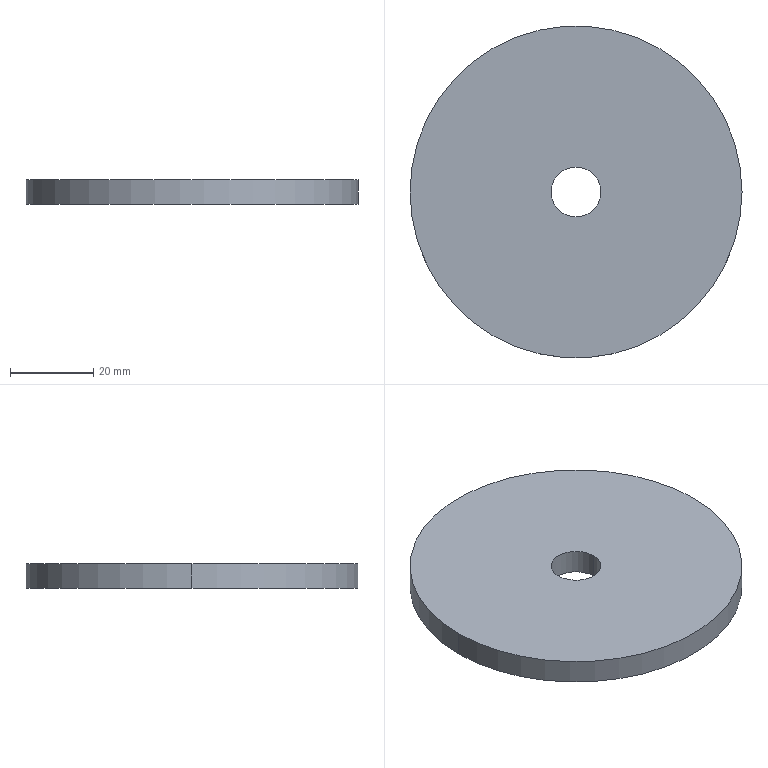Part | SolidWorks | features FlatPattern 1, SMBaseFlange 1, SheetMetal 1 | 1 solid | 6 faces | box 80 x 80 x 6 mm | volume 29481 mm3 | cylinder 4 | plane 2 | commonest cylinder face diameters 12 x2 80 x2
STEP:
#1=CARTESIAN_POINT('',(-1066.,0.,6.));
#2=VERTEX_POINT('',#1);
#3=CARTESIAN_POINT('',(-1054.,0.,6.));
#4=VERTEX_POINT('',#3);
#5=CARTESIAN_POINT('',(-1060.,0.,6.));
#6=DIRECTION('',(0.,0.,1.));
#7=DIRECTION('',(1.,0.,0.));
#8=AXIS2_PLACEMENT_3D('',#5,#6,#7);
#9=CIRCLE('',#8,6.);
#10=EDGE_CURVE('',#2,#4,#9,.T.);
#11=ORIENTED_EDGE('',*,*,#10,.T.);
#12=CARTESIAN_POINT('',(-1054.,0.,0.));
#13=VERTEX_POINT('',#12);
#14=CARTESIAN_POINT('',(-1054.,0.,6.));
#15=DIRECTION('',(0.,0.,-1.));
#16=VECTOR('',#15,1000.);
#17=LINE('',#14,#16);
#18=EDGE_CURVE('',#4,#13,#17,.T.);
#19=ORIENTED_EDGE('',*,*,#18,.T.);
#20=CARTESIAN_POINT('',(-1066.,0.,0.));
#21=VERTEX_POINT('',#20);
#22=CARTESIAN_POINT('',(-1060.,0.,0.));
#23=DIRECTION('',(0.,0.,1.));
#24=DIRECTION('',(1.,0.,0.));
#25=AXIS2_PLACEMENT_3D('',#22,#23,#24);
#26=CIRCLE('',#25,6.);
#27=EDGE_CURVE('',#21,#13,#26,.T.);
#28=ORIENTED_EDGE('',*,*,#27,.F.);
#29=CARTESIAN_POINT('',(-1066.,0.,6.));
#30=DIRECTION('',(0.,0.,-1.));
#31=VECTOR('',#30,1000.);
#32=LINE('',#29,#31);
#33=EDGE_CURVE('',#2,#21,#32,.T.);
#34=ORIENTED_EDGE('',*,*,#33,.F.);
#35=EDGE_LOOP('',(#11,#19,#28,#34));
#36=FACE_OUTER_BOUND('',#35,.T.);
#37=CARTESIAN_POINT('',(-1060.,0.,6.));
#38=DIRECTION('',(0.,0.,-1.));
#39=DIRECTION('',(-1.,0.,0.));
#40=AXIS2_PLACEMENT_3D('',#37,#38,#39);
#41=CYLINDRICAL_SURFACE('',#40,6.);
#42=ADVANCED_FACE('',(#36),#41,.F.);
#43=CARTESIAN_POINT('',(-1020.,0.,6.));
#44=VERTEX_POINT('',#43);
#45=CARTESIAN_POINT('',(-1100.,0.,6.));
#46=VERTEX_POINT('',#45);
#47=CARTESIAN_POINT('',(-1060.,0.,6.));
#48=DIRECTION('',(0.,0.,1.));
#49=DIRECTION('',(1.,0.,0.));
#50=AXIS2_PLACEMENT_3D('',#47,#48,#49);
#51=CIRCLE('',#50,40.);
#52=EDGE_CURVE('',#44,#46,#51,.T.);
#53=ORIENTED_EDGE('',*,*,#52,.F.);
#54=CARTESIAN_POINT('',(-1020.,0.,0.));
#55=VERTEX_POINT('',#54);
#56=CARTESIAN_POINT('',(-1020.,0.,6.));
#57=DIRECTION('',(0.,0.,-1.));
#58=VECTOR('',#57,1000.);
#59=LINE('',#56,#58);
#60=EDGE_CURVE('',#44,#55,#59,.T.);
#61=ORIENTED_EDGE('',*,*,#60,.T.);
#62=CARTESIAN_POINT('',(-1100.,0.,0.));
#63=VERTEX_POINT('',#62);
#64=CARTESIAN_POINT('',(-1060.,0.,0.));
#65=DIRECTION('',(0.,0.,1.));
#66=DIRECTION('',(1.,0.,0.));
#67=AXIS2_PLACEMENT_3D('',#64,#65,#66);
#68=CIRCLE('',#67,40.);
#69=EDGE_CURVE('',#55,#63,#68,.T.);
#70=ORIENTED_EDGE('',*,*,#69,.T.);
#71=CARTESIAN_POINT('',(-1100.,0.,6.));
#72=DIRECTION('',(0.,0.,-1.));
#73=VECTOR('',#72,1000.);
#74=LINE('',#71,#73);
#75=EDGE_CURVE('',#46,#63,#74,.T.);
#76=ORIENTED_EDGE('',*,*,#75,.F.);
#77=EDGE_LOOP('',(#53,#61,#70,#76));
#78=FACE_OUTER_BOUND('',#77,.T.);
#79=CARTESIAN_POINT('',(-1060.,0.,6.));
#80=DIRECTION('',(0.,0.,-1.));
#81=DIRECTION('',(-1.,0.,0.));
#82=AXIS2_PLACEMENT_3D('',#79,#80,#81);
#83=CYLINDRICAL_SURFACE('',#82,40.);
#84=ADVANCED_FACE('',(#78),#83,.T.);
#85=CARTESIAN_POINT('',(-1060.,0.,6.));
#86=DIRECTION('',(0.,0.,1.));
#87=DIRECTION('',(1.,0.,0.));
#88=AXIS2_PLACEMENT_3D('',#85,#86,#87);
#89=CIRCLE('',#88,40.);
#90=EDGE_CURVE('',#46,#44,#89,.T.);
#91=ORIENTED_EDGE('',*,*,#90,.T.);
#92=ORIENTED_EDGE('',*,*,#52,.T.);
#93=EDGE_LOOP('',(#91,#92));
#94=FACE_OUTER_BOUND('',#93,.T.);
#95=ORIENTED_EDGE('',*,*,#10,.F.);
#96=CARTESIAN_POINT('',(-1060.,0.,6.));
#97=DIRECTION('',(0.,0.,1.));
#98=DIRECTION('',(1.,0.,0.));
#99=AXIS2_PLACEMENT_3D('',#96,#97,#98);
#100=CIRCLE('',#99,6.);
#101=EDGE_CURVE('',#4,#2,#100,.T.);
#102=ORIENTED_EDGE('',*,*,#101,.F.);
#103=EDGE_LOOP('',(#95,#102));
#104=FACE_BOUND('',#103,.T.);
#105=CARTESIAN_POINT('',(-1060.,0.,6.));
#106=DIRECTION('',(0.,0.,1.));
#107=DIRECTION('',(1.,0.,0.));
#108=AXIS2_PLACEMENT_3D('',#105,#106,#107);
#109=PLANE('',#108);
#110=ADVANCED_FACE('',(#94,#104),#109,.T.);
#111=CARTESIAN_POINT('',(-1060.,0.,0.));
#112=DIRECTION('',(0.,0.,1.));
#113=DIRECTION('',(1.,0.,0.));
#114=AXIS2_PLACEMENT_3D('',#111,#112,#113);
#115=CIRCLE('',#114,40.);
#116=EDGE_CURVE('',#63,#55,#115,.T.);
#117=ORIENTED_EDGE('',*,*,#116,.F.);
#118=ORIENTED_EDGE('',*,*,#69,.F.);
#119=EDGE_LOOP('',(#117,#118));
#120=FACE_OUTER_BOUND('',#119,.T.);
#121=ORIENTED_EDGE('',*,*,#27,.T.);
#122=CARTESIAN_POINT('',(-1060.,0.,0.));
#123=DIRECTION('',(0.,0.,1.));
#124=DIRECTION('',(1.,0.,0.));
#125=AXIS2_PLACEMENT_3D('',#122,#123,#124);
#126=CIRCLE('',#125,6.);
#127=EDGE_CURVE('',#13,#21,#126,.T.);
#128=ORIENTED_EDGE('',*,*,#127,.T.);
#129=EDGE_LOOP('',(#121,#128));
#130=FACE_BOUND('',#129,.T.);
#131=CARTESIAN_POINT('',(-1060.,0.,0.));
#132=DIRECTION('',(0.,0.,1.));
#133=DIRECTION('',(1.,0.,0.));
#134=AXIS2_PLACEMENT_3D('',#131,#132,#133);
#135=PLANE('',#134);
#136=ADVANCED_FACE('',(#120,#130),#135,.F.);
#137=ORIENTED_EDGE('',*,*,#60,.F.);
#138=ORIENTED_EDGE('',*,*,#90,.F.);
#139=ORIENTED_EDGE('',*,*,#75,.T.);
#140=ORIENTED_EDGE('',*,*,#116,.T.);
#141=EDGE_LOOP('',(#137,#138,#139,#140));
#142=FACE_OUTER_BOUND('',#141,.T.);
#143=CARTESIAN_POINT('',(-1060.,0.,6.));
#144=DIRECTION('',(0.,0.,-1.));
#145=DIRECTION('',(-1.,0.,0.));
#146=AXIS2_PLACEMENT_3D('',#143,#144,#145);
#147=CYLINDRICAL_SURFACE('',#146,40.);
#148=ADVANCED_FACE('',(#142),#147,.T.);
#149=ORIENTED_EDGE('',*,*,#18,.F.);
#150=ORIENTED_EDGE('',*,*,#101,.T.);
#151=ORIENTED_EDGE('',*,*,#33,.T.);
#152=ORIENTED_EDGE('',*,*,#127,.F.);
#153=EDGE_LOOP('',(#149,#150,#151,#152));
#154=FACE_OUTER_BOUND('',#153,.T.);
#155=CARTESIAN_POINT('',(-1060.,0.,6.));
#156=DIRECTION('',(0.,0.,-1.));
#157=DIRECTION('',(-1.,0.,0.));
#158=AXIS2_PLACEMENT_3D('',#155,#156,#157);
#159=CYLINDRICAL_SURFACE('',#158,6.);
#160=ADVANCED_FACE('',(#154),#159,.F.);
#161=CLOSED_SHELL('',(#42,#84,#110,#136,#148,#160));
#162=MANIFOLD_SOLID_BREP('',#161);
#163=CARTESIAN_POINT('',(0.,0.,0.));
#164=DIRECTION('',(0.,0.,1.));
#165=DIRECTION('',(1.,0.,0.));
#166=AXIS2_PLACEMENT_3D('',#163,#164,#165);
#167=(LENGTH_UNIT()NAMED_UNIT(*)SI_UNIT(.MILLI.,.METRE.));
#168=UNCERTAINTY_MEASURE_WITH_UNIT(LENGTH_MEASURE(0.00001),#167,'','');
#169=(NAMED_UNIT(*)PLANE_ANGLE_UNIT()SI_UNIT($,.RADIAN.));
#170=(NAMED_UNIT(*)SI_UNIT($,.STERADIAN.)SOLID_ANGLE_UNIT());
#171=(GEOMETRIC_REPRESENTATION_CONTEXT(3)GLOBAL_UNCERTAINTY_ASSIGNED_CONTEXT((#168))GLOBAL_UNIT_ASSIGNED_CONTEXT((#167,#169,#170))REPRESENTATION_CONTEXT('',''));
#172=ADVANCED_BREP_SHAPE_REPRESENTATION('',(#162,#166),#171);